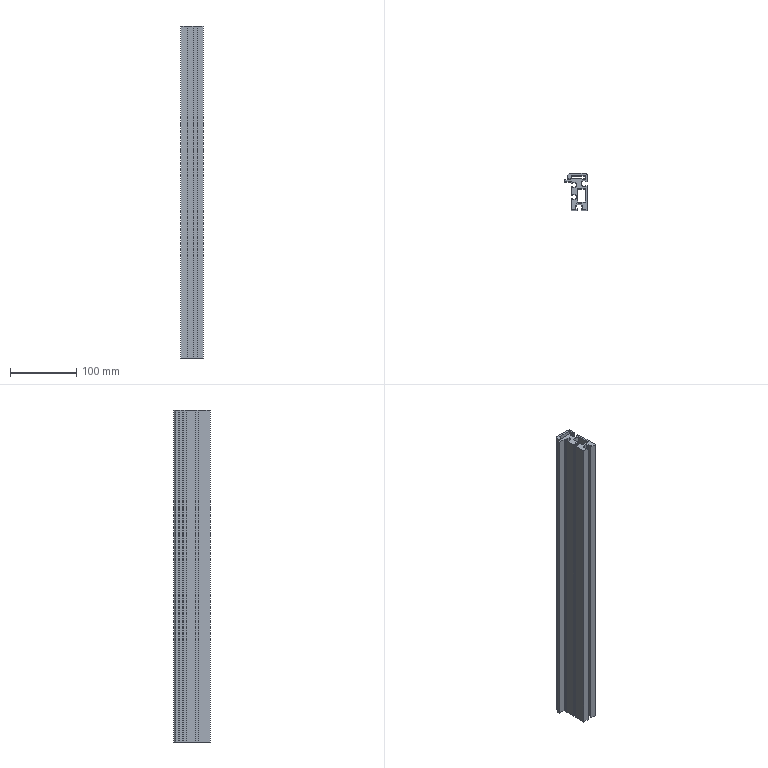Part | SolidWorks | features Extrusion 1, ICE 1 | 1 solid | 70 faces | box 33.5 x 55 x 500 mm | volume 409209 mm3 | plane 69 | cylinder 1 | commonest cylinder face diameters 6 x1